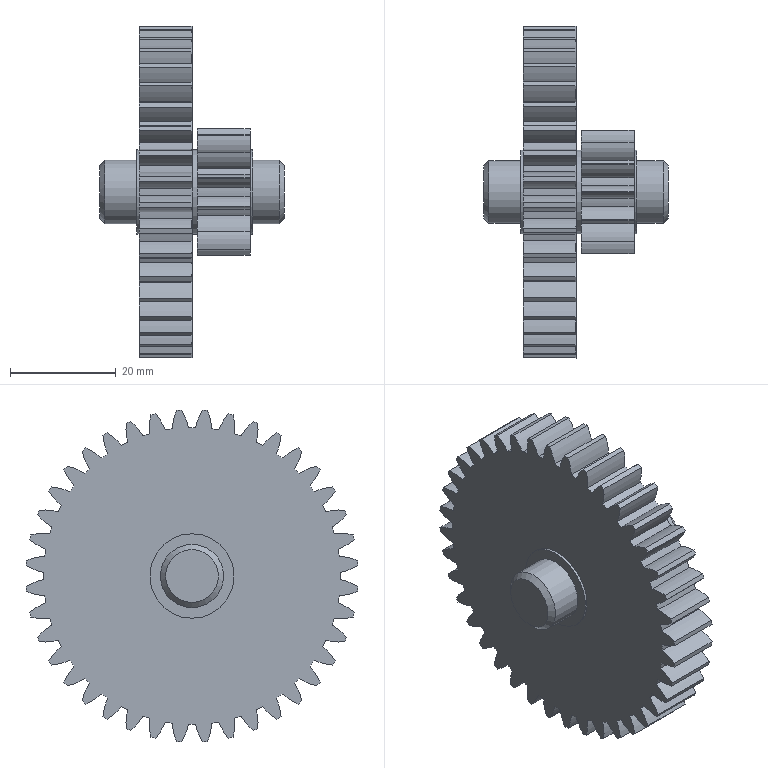Part | NX | features BREP 1 | 1 solid | 231 faces | box 35 x 62.873 x 62.873 mm | volume 32814 mm3 | cylinder 221 | plane 8 | cone 2 | commonest cylinder face diameters 24 x94 56.248 x40 63 x40 8.391 x14 8.4 x14 17.248 x14